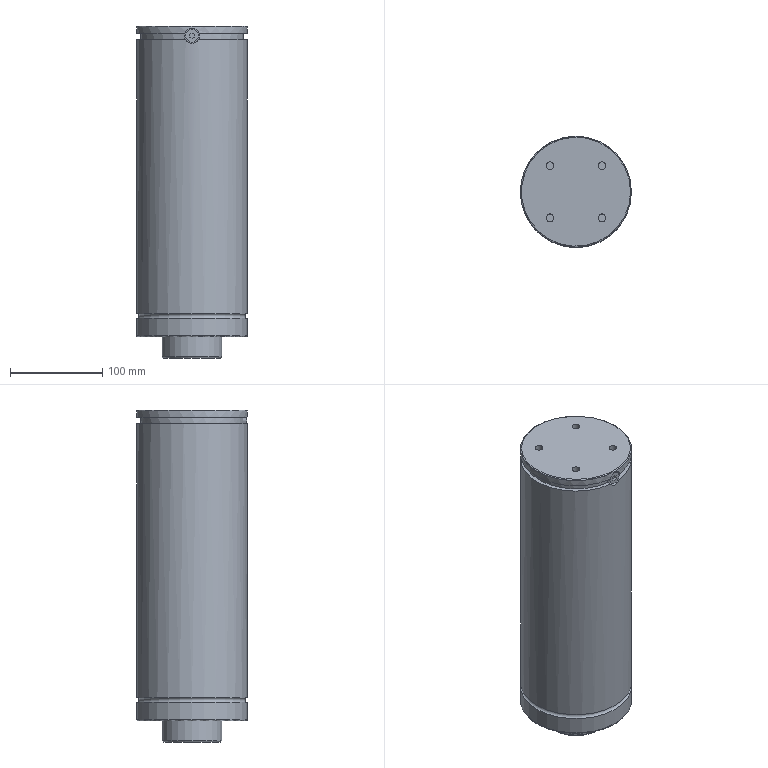Part | NX | features 1 2 | 1 solid | 38 faces | box 120.2 x 120.2 x 360 mm | volume 3879845 mm3 | plane 19 | cylinder 13 | torus 4 | cone 2 | commonest cylinder face diameters 8.4 x4 120.2 x3 6.6 x1 10 x1 14 x1 16.4 x1
STEP:
#1=CARTESIAN_POINT('',(2190.1,265.,32.15));
#2=VERTEX_POINT('',#1);
#3=CARTESIAN_POINT('',(2130.,265.,32.15));
#4=DIRECTION('',(0.,0.,1.));
#5=DIRECTION('',(1.,0.,0.));
#6=AXIS2_PLACEMENT_3D('',#3,#4,#5);
#7=CIRCLE('',#6,60.1);
#8=EDGE_CURVE('',#2,#2,#7,.T.);
#9=ORIENTED_EDGE('',*,*,#8,.F.);
#10=EDGE_LOOP('',(#9));
#11=FACE_BOUND('',#10,.T.);
#12=CARTESIAN_POINT('',(2190.1,265.,26.85));
#13=VERTEX_POINT('',#12);
#14=CARTESIAN_POINT('',(2130.,265.,26.85));
#15=DIRECTION('',(0.,0.,1.));
#16=DIRECTION('',(1.,0.,0.));
#17=AXIS2_PLACEMENT_3D('',#14,#15,#16);
#18=CIRCLE('',#17,60.1);
#19=EDGE_CURVE('',#13,#13,#18,.T.);
#20=ORIENTED_EDGE('',*,*,#19,.T.);
#21=EDGE_LOOP('',(#20));
#22=FACE_BOUND('',#21,.T.);
#23=CARTESIAN_POINT('',(2130.,265.,29.5));
#24=DIRECTION('',(0.,0.,-1.));
#25=DIRECTION('',(0.,-1.,0.));
#26=AXIS2_PLACEMENT_3D('',#23,#24,#25);
#27=TOROIDAL_SURFACE('',#26,60.1,2.65);
#28=ADVANCED_FACE('',(#11,#22),#27,.F.);
#29=CARTESIAN_POINT('',(2190.1,265.,8.));
#30=VERTEX_POINT('',#29);
#31=CARTESIAN_POINT('',(2130.,265.,8.));
#32=DIRECTION('',(0.,0.,1.));
#33=DIRECTION('',(1.,0.,0.));
#34=AXIS2_PLACEMENT_3D('',#31,#32,#33);
#35=CIRCLE('',#34,60.1);
#36=EDGE_CURVE('',#30,#30,#35,.T.);
#37=ORIENTED_EDGE('',*,*,#36,.F.);
#38=EDGE_LOOP('',(#37));
#39=FACE_BOUND('',#38,.T.);
#40=CARTESIAN_POINT('',(2189.1,265.,7.));
#41=VERTEX_POINT('',#40);
#42=CARTESIAN_POINT('',(2130.,265.,7.));
#43=DIRECTION('',(0.,0.,1.));
#44=DIRECTION('',(1.,0.,0.));
#45=AXIS2_PLACEMENT_3D('',#42,#43,#44);
#46=CIRCLE('',#45,59.1);
#47=EDGE_CURVE('',#41,#41,#46,.T.);
#48=ORIENTED_EDGE('',*,*,#47,.T.);
#49=EDGE_LOOP('',(#48));
#50=FACE_BOUND('',#49,.T.);
#51=CARTESIAN_POINT('',(2130.,265.,8.));
#52=DIRECTION('',(0.,0.,-1.));
#53=DIRECTION('',(0.,-1.,0.));
#54=AXIS2_PLACEMENT_3D('',#51,#52,#53);
#55=TOROIDAL_SURFACE('',#54,59.1,1.);
#56=ADVANCED_FACE('',(#39,#50),#55,.T.);
#57=ORIENTED_EDGE('',*,*,#19,.F.);
#58=EDGE_LOOP('',(#57));
#59=FACE_BOUND('',#58,.T.);
#60=ORIENTED_EDGE('',*,*,#36,.T.);
#61=EDGE_LOOP('',(#60));
#62=FACE_BOUND('',#61,.T.);
#63=CARTESIAN_POINT('',(2130.,265.,17.425));
#64=DIRECTION('',(0.,0.,1.));
#65=DIRECTION('',(0.,1.,0.));
#66=AXIS2_PLACEMENT_3D('',#63,#64,#65);
#67=CYLINDRICAL_SURFACE('',#66,60.1);
#68=ADVANCED_FACE('',(#59,#62),#67,.T.);
#69=CARTESIAN_POINT('',(2136.855,209.623,329.));
#70=VERTEX_POINT('',#69);
#71=CARTESIAN_POINT('',(2123.145,209.623,329.));
#72=VERTEX_POINT('',#71);
#73=CARTESIAN_POINT('',(2130.,265.,329.));
#74=DIRECTION('',(0.,0.,1.));
#75=DIRECTION('',(1.,0.,0.));
#76=AXIS2_PLACEMENT_3D('',#73,#74,#75);
#77=CIRCLE('',#76,55.8);
#78=EDGE_CURVE('',#70,#72,#77,.T.);
#79=ORIENTED_EDGE('',*,*,#78,.T.);
#80=CARTESIAN_POINT('',(2122.19,209.749,336.));
#81=VERTEX_POINT('',#80);
#82=CARTESIAN_POINT('',(2122.19,209.749,336.));
#83=CARTESIAN_POINT('',(2121.442,209.855,333.663));
#84=CARTESIAN_POINT('',(2121.8,209.789,331.049));
#85=CARTESIAN_POINT('',(2123.145,209.623,329.));
#86=B_SPLINE_CURVE_WITH_KNOTS('',3,(#82,#83,#84,#85),.UNSPECIFIED.,.F.,.F.,(4,4),(0.,0.007265),.UNSPECIFIED.);
#87=EDGE_CURVE('',#81,#72,#86,.T.);
#88=ORIENTED_EDGE('',*,*,#87,.F.);
#89=CARTESIAN_POINT('',(2137.81,209.749,336.));
#90=VERTEX_POINT('',#89);
#91=CARTESIAN_POINT('',(2130.,265.,336.));
#92=DIRECTION('',(0.,0.,1.));
#93=DIRECTION('',(1.,0.,0.));
#94=AXIS2_PLACEMENT_3D('',#91,#92,#93);
#95=CIRCLE('',#94,55.8);
#96=EDGE_CURVE('',#90,#81,#95,.T.);
#97=ORIENTED_EDGE('',*,*,#96,.F.);
#98=CARTESIAN_POINT('',(2136.855,209.623,329.));
#99=CARTESIAN_POINT('',(2138.2,209.789,331.049));
#100=CARTESIAN_POINT('',(2138.558,209.855,333.663));
#101=CARTESIAN_POINT('',(2137.81,209.749,336.));
#102=B_SPLINE_CURVE_WITH_KNOTS('',3,(#98,#99,#100,#101),.UNSPECIFIED.,.F.,.F.,(4,4),(0.,0.007265),.UNSPECIFIED.);
#103=EDGE_CURVE('',#70,#90,#102,.T.);
#104=ORIENTED_EDGE('',*,*,#103,.F.);
#105=EDGE_LOOP('',(#79,#88,#97,#104));
#106=FACE_BOUND('',#105,.T.);
#107=CARTESIAN_POINT('',(2130.,265.,332.5));
#108=DIRECTION('',(0.,0.,1.));
#109=DIRECTION('',(0.,1.,0.));
#110=AXIS2_PLACEMENT_3D('',#107,#108,#109);
#111=CYLINDRICAL_SURFACE('',#110,55.8);
#112=ADVANCED_FACE('',(#106),#111,.T.);
#113=CARTESIAN_POINT('',(2190.1,265.,343.));
#114=VERTEX_POINT('',#113);
#115=CARTESIAN_POINT('',(2130.,265.,343.));
#116=DIRECTION('',(0.,0.,1.));
#117=DIRECTION('',(1.,0.,0.));
#118=AXIS2_PLACEMENT_3D('',#115,#116,#117);
#119=CIRCLE('',#118,60.1);
#120=EDGE_CURVE('',#114,#114,#119,.T.);
#121=ORIENTED_EDGE('',*,*,#120,.F.);
#122=EDGE_LOOP('',(#121));
#123=FACE_BOUND('',#122,.T.);
#124=CARTESIAN_POINT('',(2137.81,205.41,336.));
#125=VERTEX_POINT('',#124);
#126=CARTESIAN_POINT('',(2122.19,205.41,336.));
#127=VERTEX_POINT('',#126);
#128=CARTESIAN_POINT('',(2130.,265.,336.));
#129=DIRECTION('',(0.,0.,1.));
#130=DIRECTION('',(1.,0.,0.));
#131=AXIS2_PLACEMENT_3D('',#128,#129,#130);
#132=CIRCLE('',#131,60.1);
#133=EDGE_CURVE('',#125,#127,#132,.T.);
#134=ORIENTED_EDGE('',*,*,#133,.T.);
#135=CARTESIAN_POINT('',(2137.81,205.41,336.));
#136=CARTESIAN_POINT('',(2137.279,205.34,337.657));
#137=CARTESIAN_POINT('',(2135.182,205.071,340.559));
#138=CARTESIAN_POINT('',(2129.995,204.815,342.267));
#139=CARTESIAN_POINT('',(2124.839,205.069,340.572));
#140=CARTESIAN_POINT('',(2122.721,205.34,337.657));
#141=CARTESIAN_POINT('',(2122.19,205.41,336.));
#142=B_SPLINE_CURVE_WITH_KNOTS('',3,(#135,#136,#137,#138,#139,#140,#141),.UNSPECIFIED.,.F.,.F.,(4,1,1,1,4),(-0.0103,-0.005148,-0.000000175,0.005148,0.0103),.UNSPECIFIED.);
#143=EDGE_CURVE('',#125,#127,#142,.T.);
#144=ORIENTED_EDGE('',*,*,#143,.F.);
#145=EDGE_LOOP('',(#134,#144));
#146=FACE_BOUND('',#145,.T.);
#147=CARTESIAN_POINT('',(2130.,265.,339.5));
#148=DIRECTION('',(0.,0.,1.));
#149=DIRECTION('',(0.,1.,0.));
#150=AXIS2_PLACEMENT_3D('',#147,#148,#149);
#151=CYLINDRICAL_SURFACE('',#150,60.1);
#152=ADVANCED_FACE('',(#123,#146),#151,.T.);
#153=CARTESIAN_POINT('',(2189.1,265.,344.));
#154=VERTEX_POINT('',#153);
#155=CARTESIAN_POINT('',(2130.,265.,344.));
#156=DIRECTION('',(0.,0.,1.));
#157=DIRECTION('',(1.,0.,0.));
#158=AXIS2_PLACEMENT_3D('',#155,#156,#157);
#159=CIRCLE('',#158,59.1);
#160=EDGE_CURVE('',#154,#154,#159,.T.);
#161=ORIENTED_EDGE('',*,*,#160,.F.);
#162=EDGE_LOOP('',(#161));
#163=FACE_BOUND('',#162,.T.);
#164=ORIENTED_EDGE('',*,*,#120,.T.);
#165=EDGE_LOOP('',(#164));
#166=FACE_BOUND('',#165,.T.);
#167=CARTESIAN_POINT('',(2130.,265.,343.));
#168=DIRECTION('',(0.,0.,-1.));
#169=DIRECTION('',(0.,-1.,0.));
#170=AXIS2_PLACEMENT_3D('',#167,#168,#169);
#171=TOROIDAL_SURFACE('',#170,59.1,1.);
#172=ADVANCED_FACE('',(#163,#166),#171,.T.);
#173=CARTESIAN_POINT('',(2162.5,265.,-14.5));
#174=VERTEX_POINT('',#173);
#175=CARTESIAN_POINT('',(2130.,265.,-14.5));
#176=DIRECTION('',(0.,0.,1.));
#177=DIRECTION('',(1.,0.,0.));
#178=AXIS2_PLACEMENT_3D('',#175,#176,#177);
#179=CIRCLE('',#178,32.5);
#180=EDGE_CURVE('',#174,#174,#179,.T.);
#181=ORIENTED_EDGE('',*,*,#180,.F.);
#182=EDGE_LOOP('',(#181));
#183=FACE_BOUND('',#182,.T.);
#184=CARTESIAN_POINT('',(2161.,265.,-16.));
#185=VERTEX_POINT('',#184);
#186=CARTESIAN_POINT('',(2130.,265.,-16.));
#187=DIRECTION('',(0.,0.,1.));
#188=DIRECTION('',(1.,0.,0.));
#189=AXIS2_PLACEMENT_3D('',#186,#187,#188);
#190=CIRCLE('',#189,31.);
#191=EDGE_CURVE('',#185,#185,#190,.T.);
#192=ORIENTED_EDGE('',*,*,#191,.T.);
#193=EDGE_LOOP('',(#192));
#194=FACE_BOUND('',#193,.T.);
#195=CARTESIAN_POINT('',(2130.,265.,-14.5));
#196=DIRECTION('',(0.,0.,-1.));
#197=DIRECTION('',(0.,-1.,0.));
#198=AXIS2_PLACEMENT_3D('',#195,#196,#197);
#199=TOROIDAL_SURFACE('',#198,31.,1.5);
#200=ADVANCED_FACE('',(#183,#194),#199,.T.);
#201=CARTESIAN_POINT('',(2162.5,265.,7.));
#202=VERTEX_POINT('',#201);
#203=CARTESIAN_POINT('',(2130.,265.,7.));
#204=DIRECTION('',(0.,0.,-1.));
#205=DIRECTION('',(1.,0.,0.));
#206=AXIS2_PLACEMENT_3D('',#203,#204,#205);
#207=CIRCLE('',#206,32.5);
#208=EDGE_CURVE('',#202,#202,#207,.T.);
#209=ORIENTED_EDGE('',*,*,#208,.T.);
#210=EDGE_LOOP('',(#209));
#211=FACE_BOUND('',#210,.T.);
#212=ORIENTED_EDGE('',*,*,#180,.T.);
#213=EDGE_LOOP('',(#212));
#214=FACE_BOUND('',#213,.T.);
#215=CARTESIAN_POINT('',(2130.,265.,-3.75));
#216=DIRECTION('',(0.,0.,1.));
#217=DIRECTION('',(0.,1.,0.));
#218=AXIS2_PLACEMENT_3D('',#215,#216,#217);
#219=CYLINDRICAL_SURFACE('',#218,32.5);
#220=ADVANCED_FACE('',(#211,#214),#219,.T.);
#221=CARTESIAN_POINT('',(2136.855,205.292,329.));
#222=VERTEX_POINT('',#221);
#223=CARTESIAN_POINT('',(2123.145,205.292,329.));
#224=VERTEX_POINT('',#223);
#225=CARTESIAN_POINT('',(2130.,265.,329.));
#226=DIRECTION('',(0.,0.,1.));
#227=DIRECTION('',(1.,0.,0.));
#228=AXIS2_PLACEMENT_3D('',#225,#226,#227);
#229=CIRCLE('',#228,60.1);
#230=EDGE_CURVE('',#222,#224,#229,.T.);
#231=ORIENTED_EDGE('',*,*,#230,.F.);
#232=CARTESIAN_POINT('',(2123.145,205.292,329.));
#233=CARTESIAN_POINT('',(2123.894,205.206,327.859));
#234=CARTESIAN_POINT('',(2125.933,205.,325.992));
#235=CARTESIAN_POINT('',(2130.001,204.85,324.954));
#236=CARTESIAN_POINT('',(2134.063,205.,325.991));
#237=CARTESIAN_POINT('',(2136.106,205.206,327.859));
#238=CARTESIAN_POINT('',(2136.855,205.292,329.));
#239=B_SPLINE_CURVE_WITH_KNOTS('',3,(#232,#233,#234,#235,#236,#237,#238),.UNSPECIFIED.,.F.,.F.,(4,1,1,1,4),(-0.008087,-0.004043,-0.000000027,0.004043,0.008087),.UNSPECIFIED.);
#240=EDGE_CURVE('',#224,#222,#239,.T.);
#241=ORIENTED_EDGE('',*,*,#240,.F.);
#242=EDGE_LOOP('',(#231,#241));
#243=FACE_BOUND('',#242,.T.);
#244=ORIENTED_EDGE('',*,*,#8,.T.);
#245=EDGE_LOOP('',(#244));
#246=FACE_BOUND('',#245,.T.);
#247=CARTESIAN_POINT('',(2130.,265.,180.575));
#248=DIRECTION('',(0.,0.,1.));
#249=DIRECTION('',(0.,1.,0.));
#250=AXIS2_PLACEMENT_3D('',#247,#248,#249);
#251=CYLINDRICAL_SURFACE('',#250,60.1);
#252=ADVANCED_FACE('',(#243,#246),#251,.T.);
#253=CARTESIAN_POINT('',(2138.2,210.9,333.5));
#254=VERTEX_POINT('',#253);
#255=CARTESIAN_POINT('',(2130.,210.9,333.5));
#256=DIRECTION('',(0.,1.,0.));
#257=DIRECTION('',(1.,0.,0.));
#258=AXIS2_PLACEMENT_3D('',#255,#256,#257);
#259=CIRCLE('',#258,8.2);
#260=EDGE_CURVE('',#254,#254,#259,.T.);
#261=ORIENTED_EDGE('',*,*,#260,.T.);
#262=EDGE_LOOP('',(#261));
#263=FACE_BOUND('',#262,.T.);
#264=ORIENTED_EDGE('',*,*,#103,.T.);
#265=CARTESIAN_POINT('',(2137.81,207.9,336.));
#266=DIRECTION('',(0.,-1.,0.));
#267=VECTOR('',#266,1000.);
#268=LINE('',#265,#267);
#269=EDGE_CURVE('',#90,#125,#268,.T.);
#270=ORIENTED_EDGE('',*,*,#269,.T.);
#271=ORIENTED_EDGE('',*,*,#143,.T.);
#272=CARTESIAN_POINT('',(2122.19,207.9,336.));
#273=DIRECTION('',(0.,1.,0.));
#274=VECTOR('',#273,1000.);
#275=LINE('',#272,#274);
#276=EDGE_CURVE('',#127,#81,#275,.T.);
#277=ORIENTED_EDGE('',*,*,#276,.T.);
#278=ORIENTED_EDGE('',*,*,#87,.T.);
#279=CARTESIAN_POINT('',(2123.145,207.9,329.));
#280=DIRECTION('',(0.,-1.,0.));
#281=VECTOR('',#280,1000.);
#282=LINE('',#279,#281);
#283=EDGE_CURVE('',#72,#224,#282,.T.);
#284=ORIENTED_EDGE('',*,*,#283,.T.);
#285=ORIENTED_EDGE('',*,*,#240,.T.);
#286=CARTESIAN_POINT('',(2136.855,207.9,329.));
#287=DIRECTION('',(0.,1.,0.));
#288=VECTOR('',#287,1000.);
#289=LINE('',#286,#288);
#290=EDGE_CURVE('',#222,#70,#289,.T.);
#291=ORIENTED_EDGE('',*,*,#290,.T.);
#292=EDGE_LOOP('',(#264,#270,#271,#277,#278,#284,#285,#291));
#293=FACE_BOUND('',#292,.T.);
#294=CARTESIAN_POINT('',(2130.,204.9,333.5));
#295=DIRECTION('',(0.,-1.,0.));
#296=DIRECTION('',(1.,0.,0.));
#297=AXIS2_PLACEMENT_3D('',#294,#295,#296);
#298=CYLINDRICAL_SURFACE('',#297,8.2);
#299=ADVANCED_FACE('',(#263,#293),#298,.F.);
#300=CARTESIAN_POINT('',(2105.916,293.284,324.));
#301=VERTEX_POINT('',#300);
#302=CARTESIAN_POINT('',(2101.716,293.284,324.));
#303=DIRECTION('',(0.,0.,-1.));
#304=DIRECTION('',(1.,0.,0.));
#305=AXIS2_PLACEMENT_3D('',#302,#303,#304);
#306=CIRCLE('',#305,4.2);
#307=EDGE_CURVE('',#301,#301,#306,.T.);
#308=ORIENTED_EDGE('',*,*,#307,.T.);
#309=EDGE_LOOP('',(#308));
#310=FACE_BOUND('',#309,.T.);
#311=CARTESIAN_POINT('',(2105.916,293.284,344.));
#312=VERTEX_POINT('',#311);
#313=CARTESIAN_POINT('',(2101.716,293.284,344.));
#314=DIRECTION('',(0.,0.,1.));
#315=DIRECTION('',(1.,0.,0.));
#316=AXIS2_PLACEMENT_3D('',#313,#314,#315);
#317=CIRCLE('',#316,4.2);
#318=EDGE_CURVE('',#312,#312,#317,.T.);
#319=ORIENTED_EDGE('',*,*,#318,.T.);
#320=EDGE_LOOP('',(#319));
#321=FACE_BOUND('',#320,.T.);
#322=CARTESIAN_POINT('',(2101.716,293.284,344.));
#323=DIRECTION('',(0.,0.,1.));
#324=DIRECTION('',(0.,1.,0.));
#325=AXIS2_PLACEMENT_3D('',#322,#323,#324);
#326=CYLINDRICAL_SURFACE('',#325,4.2);
#327=ADVANCED_FACE('',(#310,#321),#326,.F.);
#328=CARTESIAN_POINT('',(2162.484,293.284,324.));
#329=VERTEX_POINT('',#328);
#330=CARTESIAN_POINT('',(2158.284,293.284,324.));
#331=DIRECTION('',(0.,0.,-1.));
#332=DIRECTION('',(1.,0.,0.));
#333=AXIS2_PLACEMENT_3D('',#330,#331,#332);
#334=CIRCLE('',#333,4.2);
#335=EDGE_CURVE('',#329,#329,#334,.T.);
#336=ORIENTED_EDGE('',*,*,#335,.T.);
#337=EDGE_LOOP('',(#336));
#338=FACE_BOUND('',#337,.T.);
#339=CARTESIAN_POINT('',(2162.484,293.284,344.));
#340=VERTEX_POINT('',#339);
#341=CARTESIAN_POINT('',(2158.284,293.284,344.));
#342=DIRECTION('',(0.,0.,1.));
#343=DIRECTION('',(1.,0.,0.));
#344=AXIS2_PLACEMENT_3D('',#341,#342,#343);
#345=CIRCLE('',#344,4.2);
#346=EDGE_CURVE('',#340,#340,#345,.T.);
#347=ORIENTED_EDGE('',*,*,#346,.T.);
#348=EDGE_LOOP('',(#347));
#349=FACE_BOUND('',#348,.T.);
#350=CARTESIAN_POINT('',(2158.284,293.284,344.));
#351=DIRECTION('',(0.,0.,1.));
#352=DIRECTION('',(0.,1.,0.));
#353=AXIS2_PLACEMENT_3D('',#350,#351,#352);
#354=CYLINDRICAL_SURFACE('',#353,4.2);
#355=ADVANCED_FACE('',(#338,#349),#354,.F.);
#356=CARTESIAN_POINT('',(2162.484,236.716,324.));
#357=VERTEX_POINT('',#356);
#358=CARTESIAN_POINT('',(2158.284,236.716,324.));
#359=DIRECTION('',(0.,0.,-1.));
#360=DIRECTION('',(1.,0.,0.));
#361=AXIS2_PLACEMENT_3D('',#358,#359,#360);
#362=CIRCLE('',#361,4.2);
#363=EDGE_CURVE('',#357,#357,#362,.T.);
#364=ORIENTED_EDGE('',*,*,#363,.T.);
#365=EDGE_LOOP('',(#364));
#366=FACE_BOUND('',#365,.T.);
#367=CARTESIAN_POINT('',(2162.484,236.716,344.));
#368=VERTEX_POINT('',#367);
#369=CARTESIAN_POINT('',(2158.284,236.716,344.));
#370=DIRECTION('',(0.,0.,1.));
#371=DIRECTION('',(1.,0.,0.));
#372=AXIS2_PLACEMENT_3D('',#369,#370,#371);
#373=CIRCLE('',#372,4.2);
#374=EDGE_CURVE('',#368,#368,#373,.T.);
#375=ORIENTED_EDGE('',*,*,#374,.T.);
#376=EDGE_LOOP('',(#375));
#377=FACE_BOUND('',#376,.T.);
#378=CARTESIAN_POINT('',(2158.284,236.716,344.));
#379=DIRECTION('',(0.,0.,1.));
#380=DIRECTION('',(0.,1.,0.));
#381=AXIS2_PLACEMENT_3D('',#378,#379,#380);
#382=CYLINDRICAL_SURFACE('',#381,4.2);
#383=ADVANCED_FACE('',(#366,#377),#382,.F.);
#384=CARTESIAN_POINT('',(2105.916,236.716,324.));
#385=VERTEX_POINT('',#384);
#386=CARTESIAN_POINT('',(2101.716,236.716,324.));
#387=DIRECTION('',(0.,0.,-1.));
#388=DIRECTION('',(1.,0.,0.));
#389=AXIS2_PLACEMENT_3D('',#386,#387,#388);
#390=CIRCLE('',#389,4.2);
#391=EDGE_CURVE('',#385,#385,#390,.T.);
#392=ORIENTED_EDGE('',*,*,#391,.T.);
#393=EDGE_LOOP('',(#392));
#394=FACE_BOUND('',#393,.T.);
#395=CARTESIAN_POINT('',(2105.916,236.716,344.));
#396=VERTEX_POINT('',#395);
#397=CARTESIAN_POINT('',(2101.716,236.716,344.));
#398=DIRECTION('',(0.,0.,1.));
#399=DIRECTION('',(1.,0.,0.));
#400=AXIS2_PLACEMENT_3D('',#397,#398,#399);
#401=CIRCLE('',#400,4.2);
#402=EDGE_CURVE('',#396,#396,#401,.T.);
#403=ORIENTED_EDGE('',*,*,#402,.T.);
#404=EDGE_LOOP('',(#403));
#405=FACE_BOUND('',#404,.T.);
#406=CARTESIAN_POINT('',(2101.716,236.716,344.));
#407=DIRECTION('',(0.,0.,1.));
#408=DIRECTION('',(0.,1.,0.));
#409=AXIS2_PLACEMENT_3D('',#406,#407,#408);
#410=CYLINDRICAL_SURFACE('',#409,4.2);
#411=ADVANCED_FACE('',(#394,#405),#410,.F.);
#412=CARTESIAN_POINT('',(2137.,210.9,333.5));
#413=VERTEX_POINT('',#412);
#414=CARTESIAN_POINT('',(2130.,210.9,333.5));
#415=DIRECTION('',(0.,-1.,0.));
#416=DIRECTION('',(1.,0.,0.));
#417=AXIS2_PLACEMENT_3D('',#414,#415,#416);
#418=CIRCLE('',#417,7.);
#419=EDGE_CURVE('',#413,#413,#418,.T.);
#420=ORIENTED_EDGE('',*,*,#419,.T.);
#421=EDGE_LOOP('',(#420));
#422=FACE_BOUND('',#421,.T.);
#423=CARTESIAN_POINT('',(2137.,205.9,333.5));
#424=VERTEX_POINT('',#423);
#425=CARTESIAN_POINT('',(2130.,205.9,333.5));
#426=DIRECTION('',(0.,-1.,0.));
#427=DIRECTION('',(1.,0.,0.));
#428=AXIS2_PLACEMENT_3D('',#425,#426,#427);
#429=CIRCLE('',#428,7.);
#430=EDGE_CURVE('',#424,#424,#429,.T.);
#431=ORIENTED_EDGE('',*,*,#430,.F.);
#432=EDGE_LOOP('',(#431));
#433=FACE_BOUND('',#432,.T.);
#434=CARTESIAN_POINT('',(2130.,265.,333.5));
#435=DIRECTION('',(0.,1.,0.));
#436=DIRECTION('',(-1.,0.,0.));
#437=AXIS2_PLACEMENT_3D('',#434,#435,#436);
#438=CYLINDRICAL_SURFACE('',#437,7.);
#439=ADVANCED_FACE('',(#422,#433),#438,.T.);
#440=CARTESIAN_POINT('',(2130.,270.5,-16.));
#441=VERTEX_POINT('',#440);
#442=CARTESIAN_POINT('',(2130.,265.,-16.));
#443=DIRECTION('',(0.,0.,-1.));
#444=DIRECTION('',(0.,1.,0.));
#445=AXIS2_PLACEMENT_3D('',#442,#443,#444);
#446=CIRCLE('',#445,5.5);
#447=EDGE_CURVE('',#441,#441,#446,.T.);
#448=ORIENTED_EDGE('',*,*,#447,.T.);
#449=EDGE_LOOP('',(#448));
#450=FACE_BOUND('',#449,.T.);
#451=CARTESIAN_POINT('',(2130.,270.,-15.));
#452=VERTEX_POINT('',#451);
#453=CARTESIAN_POINT('',(2130.,265.,-15.));
#454=DIRECTION('',(0.,0.,1.));
#455=DIRECTION('',(0.,1.,0.));
#456=AXIS2_PLACEMENT_3D('',#453,#454,#455);
#457=CIRCLE('',#456,5.);
#458=EDGE_CURVE('',#452,#452,#457,.T.);
#459=ORIENTED_EDGE('',*,*,#458,.T.);
#460=EDGE_LOOP('',(#459));
#461=FACE_BOUND('',#460,.T.);
#462=CARTESIAN_POINT('',(2130.,265.,-15.5));
#463=DIRECTION('',(0.,0.,-1.));
#464=DIRECTION('',(0.,-1.,0.));
#465=AXIS2_PLACEMENT_3D('',#462,#463,#464);
#466=CONICAL_SURFACE('',#465,5.25,0.4636);
#467=ADVANCED_FACE('',(#450,#461),#466,.F.);
#468=ORIENTED_EDGE('',*,*,#458,.F.);
#469=EDGE_LOOP('',(#468));
#470=FACE_BOUND('',#469,.T.);
#471=CARTESIAN_POINT('',(2130.,270.,-10.));
#472=VERTEX_POINT('',#471);
#473=CARTESIAN_POINT('',(2130.,265.,-10.));
#474=DIRECTION('',(0.,0.,1.));
#475=DIRECTION('',(0.,1.,0.));
#476=AXIS2_PLACEMENT_3D('',#473,#474,#475);
#477=CIRCLE('',#476,5.);
#478=EDGE_CURVE('',#472,#472,#477,.T.);
#479=ORIENTED_EDGE('',*,*,#478,.T.);
#480=EDGE_LOOP('',(#479));
#481=FACE_BOUND('',#480,.T.);
#482=CARTESIAN_POINT('',(2130.,265.,-12.5));
#483=DIRECTION('',(0.,0.,1.));
#484=DIRECTION('',(0.,1.,0.));
#485=AXIS2_PLACEMENT_3D('',#482,#483,#484);
#486=CYLINDRICAL_SURFACE('',#485,5.);
#487=ADVANCED_FACE('',(#470,#481),#486,.F.);
#488=CARTESIAN_POINT('',(2130.,268.3,-10.));
#489=VERTEX_POINT('',#488);
#490=CARTESIAN_POINT('',(2130.,265.,-10.));
#491=DIRECTION('',(0.,0.,1.));
#492=DIRECTION('',(0.,1.,0.));
#493=AXIS2_PLACEMENT_3D('',#490,#491,#492);
#494=CIRCLE('',#493,3.3);
#495=EDGE_CURVE('',#489,#489,#494,.T.);
#496=ORIENTED_EDGE('',*,*,#495,.F.);
#497=EDGE_LOOP('',(#496));
#498=FACE_BOUND('',#497,.T.);
#499=CARTESIAN_POINT('',(2130.,268.3,-2.));
#500=VERTEX_POINT('',#499);
#501=CARTESIAN_POINT('',(2130.,265.,-2.));
#502=DIRECTION('',(0.,0.,1.));
#503=DIRECTION('',(0.,1.,0.));
#504=AXIS2_PLACEMENT_3D('',#501,#502,#503);
#505=CIRCLE('',#504,3.3);
#506=EDGE_CURVE('',#500,#500,#505,.T.);
#507=ORIENTED_EDGE('',*,*,#506,.T.);
#508=EDGE_LOOP('',(#507));
#509=FACE_BOUND('',#508,.T.);
#510=CARTESIAN_POINT('',(2130.,265.,-6.));
#511=DIRECTION('',(0.,0.,1.));
#512=DIRECTION('',(0.,1.,0.));
#513=AXIS2_PLACEMENT_3D('',#510,#511,#512);
#514=CYLINDRICAL_SURFACE('',#513,3.3);
#515=ADVANCED_FACE('',(#498,#509),#514,.F.);
#516=CARTESIAN_POINT('',(2130.,265.,0.));
#517=VERTEX_POINT('',#516);
#518=VERTEX_LOOP('',#517);
#519=FACE_BOUND('',#518,.T.);
#520=ORIENTED_EDGE('',*,*,#506,.F.);
#521=EDGE_LOOP('',(#520));
#522=FACE_BOUND('',#521,.T.);
#523=CARTESIAN_POINT('',(2130.,265.,-1.));
#524=DIRECTION('',(0.,0.,-1.));
#525=DIRECTION('',(0.,-1.,0.));
#526=AXIS2_PLACEMENT_3D('',#523,#524,#525);
#527=CONICAL_SURFACE('',#526,1.65,1.026);
#528=ADVANCED_FACE('',(#519,#522),#527,.F.);
#529=ORIENTED_EDGE('',*,*,#478,.F.);
#530=EDGE_LOOP('',(#529));
#531=FACE_BOUND('',#530,.T.);
#532=ORIENTED_EDGE('',*,*,#495,.T.);
#533=EDGE_LOOP('',(#532));
#534=FACE_BOUND('',#533,.T.);
#535=CARTESIAN_POINT('',(2130.,269.15,-10.));
#536=DIRECTION('',(0.,0.,1.));
#537=DIRECTION('',(0.,1.,0.));
#538=AXIS2_PLACEMENT_3D('',#535,#536,#537);
#539=PLANE('',#538);
#540=ADVANCED_FACE('',(#531,#534),#539,.F.);
#541=CARTESIAN_POINT('',(2130.,205.9,330.613));
#542=VERTEX_POINT('',#541);
#543=CARTESIAN_POINT('',(2132.5,205.9,332.057));
#544=VERTEX_POINT('',#543);
#545=CARTESIAN_POINT('',(2134.148,205.9,333.008));
#546=DIRECTION('',(0.866,0.,0.5));
#547=VECTOR('',#546,1000.);
#548=LINE('',#545,#547);
#549=EDGE_CURVE('',#542,#544,#548,.T.);
#550=ORIENTED_EDGE('',*,*,#549,.T.);
#551=CARTESIAN_POINT('',(2132.5,208.9,332.057));
#552=VERTEX_POINT('',#551);
#553=CARTESIAN_POINT('',(2132.5,204.9,332.057));
#554=DIRECTION('',(0.,1.,0.));
#555=VECTOR('',#554,1000.);
#556=LINE('',#553,#555);
#557=EDGE_CURVE('',#544,#552,#556,.T.);
#558=ORIENTED_EDGE('',*,*,#557,.T.);
#559=CARTESIAN_POINT('',(2130.,208.9,330.613));
#560=VERTEX_POINT('',#559);
#561=CARTESIAN_POINT('',(2132.5,208.9,332.057));
#562=DIRECTION('',(-0.866,0.,-0.5));
#563=VECTOR('',#562,1000.);
#564=LINE('',#561,#563);
#565=EDGE_CURVE('',#552,#560,#564,.T.);
#566=ORIENTED_EDGE('',*,*,#565,.T.);
#567=CARTESIAN_POINT('',(2130.,204.9,330.613));
#568=DIRECTION('',(0.,1.,0.));
#569=VECTOR('',#568,1000.);
#570=LINE('',#567,#569);
#571=EDGE_CURVE('',#542,#560,#570,.T.);
#572=ORIENTED_EDGE('',*,*,#571,.F.);
#573=EDGE_LOOP('',(#550,#558,#566,#572));
#574=FACE_BOUND('',#573,.T.);
#575=CARTESIAN_POINT('',(2132.5,204.9,332.057));
#576=DIRECTION('',(0.5,0.,-0.866));
#577=DIRECTION('',(-0.866,0.,-0.5));
#578=AXIS2_PLACEMENT_3D('',#575,#576,#577);
#579=PLANE('',#578);
#580=ADVANCED_FACE('',(#574),#579,.F.);
#581=CARTESIAN_POINT('',(2132.5,205.9,334.943));
#582=VERTEX_POINT('',#581);
#583=CARTESIAN_POINT('',(2132.5,205.9,339.472));
#584=DIRECTION('',(0.,0.,1.));
#585=VECTOR('',#584,1000.);
#586=LINE('',#583,#585);
#587=EDGE_CURVE('',#544,#582,#586,.T.);
#588=ORIENTED_EDGE('',*,*,#587,.T.);
#589=CARTESIAN_POINT('',(2132.5,208.9,334.943));
#590=VERTEX_POINT('',#589);
#591=CARTESIAN_POINT('',(2132.5,204.9,334.943));
#592=DIRECTION('',(0.,1.,0.));
#593=VECTOR('',#592,1000.);
#594=LINE('',#591,#593);
#595=EDGE_CURVE('',#582,#590,#594,.T.);
#596=ORIENTED_EDGE('',*,*,#595,.T.);
#597=CARTESIAN_POINT('',(2132.5,208.9,334.943));
#598=DIRECTION('',(0.,0.,-1.));
#599=VECTOR('',#598,1000.);
#600=LINE('',#597,#599);
#601=EDGE_CURVE('',#590,#552,#600,.T.);
#602=ORIENTED_EDGE('',*,*,#601,.T.);
#603=ORIENTED_EDGE('',*,*,#557,.F.);
#604=EDGE_LOOP('',(#588,#596,#602,#603));
#605=FACE_BOUND('',#604,.T.);
#606=CARTESIAN_POINT('',(2132.5,204.9,334.943));
#607=DIRECTION('',(1.,0.,0.));
#608=DIRECTION('',(0.,1.,0.));
#609=AXIS2_PLACEMENT_3D('',#606,#607,#608);
#610=PLANE('',#609);
#611=ADVANCED_FACE('',(#605),#610,.F.);
#612=CARTESIAN_POINT('',(2130.,205.9,336.387));
#613=VERTEX_POINT('',#612);
#614=CARTESIAN_POINT('',(2128.352,205.9,337.338));
#615=DIRECTION('',(-0.866,0.,0.5));
#616=VECTOR('',#615,1000.);
#617=LINE('',#614,#616);
#618=EDGE_CURVE('',#582,#613,#617,.T.);
#619=ORIENTED_EDGE('',*,*,#618,.T.);
#620=CARTESIAN_POINT('',(2130.,208.9,336.387));
#621=VERTEX_POINT('',#620);
#622=CARTESIAN_POINT('',(2130.,204.9,336.387));
#623=DIRECTION('',(0.,1.,0.));
#624=VECTOR('',#623,1000.);
#625=LINE('',#622,#624);
#626=EDGE_CURVE('',#613,#621,#625,.T.);
#627=ORIENTED_EDGE('',*,*,#626,.T.);
#628=CARTESIAN_POINT('',(2130.,208.9,336.387));
#629=DIRECTION('',(0.866,0.,-0.5));
#630=VECTOR('',#629,1000.);
#631=LINE('',#628,#630);
#632=EDGE_CURVE('',#621,#590,#631,.T.);
#633=ORIENTED_EDGE('',*,*,#632,.T.);
#634=ORIENTED_EDGE('',*,*,#595,.F.);
#635=EDGE_LOOP('',(#619,#627,#633,#634));
#636=FACE_BOUND('',#635,.T.);
#637=CARTESIAN_POINT('',(2130.,204.9,336.387));
#638=DIRECTION('',(0.5,0.,0.866));
#639=DIRECTION('',(0.866,0.,-0.5));
#640=AXIS2_PLACEMENT_3D('',#637,#638,#639);
#641=PLANE('',#640);
#642=ADVANCED_FACE('',(#636),#641,.F.);
#643=CARTESIAN_POINT('',(2127.5,205.9,334.943));
#644=VERTEX_POINT('',#643);
#645=CARTESIAN_POINT('',(2130.398,205.9,336.617));
#646=DIRECTION('',(-0.866,0.,-0.5));
#647=VECTOR('',#646,1000.);
#648=LINE('',#645,#647);
#649=EDGE_CURVE('',#613,#644,#648,.T.);
#650=ORIENTED_EDGE('',*,*,#649,.T.);
#651=CARTESIAN_POINT('',(2127.5,208.9,334.943));
#652=VERTEX_POINT('',#651);
#653=CARTESIAN_POINT('',(2127.5,204.9,334.943));
#654=DIRECTION('',(0.,1.,0.));
#655=VECTOR('',#654,1000.);
#656=LINE('',#653,#655);
#657=EDGE_CURVE('',#644,#652,#656,.T.);
#658=ORIENTED_EDGE('',*,*,#657,.T.);
#659=CARTESIAN_POINT('',(2127.5,208.9,334.943));
#660=DIRECTION('',(0.866,0.,0.5));
#661=VECTOR('',#660,1000.);
#662=LINE('',#659,#661);
#663=EDGE_CURVE('',#652,#621,#662,.T.);
#664=ORIENTED_EDGE('',*,*,#663,.T.);
#665=ORIENTED_EDGE('',*,*,#626,.F.);
#666=EDGE_LOOP('',(#650,#658,#664,#665));
#667=FACE_BOUND('',#666,.T.);
#668=CARTESIAN_POINT('',(2127.5,204.9,334.943));
#669=DIRECTION('',(-0.5,0.,0.866));
#670=DIRECTION('',(0.866,0.,0.5));
#671=AXIS2_PLACEMENT_3D('',#668,#669,#670);
#672=PLANE('',#671);
#673=ADVANCED_FACE('',(#667),#672,.F.);
#674=CARTESIAN_POINT('',(2127.5,205.9,332.057));
#675=VERTEX_POINT('',#674);
#676=CARTESIAN_POINT('',(2127.102,205.9,332.287));
#677=DIRECTION('',(0.866,0.,-0.5));
#678=VECTOR('',#677,1000.);
#679=LINE('',#676,#678);
#680=EDGE_CURVE('',#675,#542,#679,.T.);
#681=ORIENTED_EDGE('',*,*,#680,.T.);
#682=ORIENTED_EDGE('',*,*,#571,.T.);
#683=CARTESIAN_POINT('',(2127.5,208.9,332.057));
#684=VERTEX_POINT('',#683);
#685=CARTESIAN_POINT('',(2130.,208.9,330.613));
#686=DIRECTION('',(-0.866,0.,0.5));
#687=VECTOR('',#686,1000.);
#688=LINE('',#685,#687);
#689=EDGE_CURVE('',#560,#684,#688,.T.);
#690=ORIENTED_EDGE('',*,*,#689,.T.);
#691=CARTESIAN_POINT('',(2127.5,204.9,332.057));
#692=DIRECTION('',(0.,1.,0.));
#693=VECTOR('',#692,1000.);
#694=LINE('',#691,#693);
#695=EDGE_CURVE('',#675,#684,#694,.T.);
#696=ORIENTED_EDGE('',*,*,#695,.F.);
#697=EDGE_LOOP('',(#681,#682,#690,#696));
#698=FACE_BOUND('',#697,.T.);
#699=CARTESIAN_POINT('',(2130.,204.9,330.613));
#700=DIRECTION('',(-0.5,0.,-0.866));
#701=DIRECTION('',(-0.866,0.,0.5));
#702=AXIS2_PLACEMENT_3D('',#699,#700,#701);
#703=PLANE('',#702);
#704=ADVANCED_FACE('',(#698),#703,.F.);
#705=CARTESIAN_POINT('',(2127.5,205.9,338.028));
#706=DIRECTION('',(0.,0.,-1.));
#707=VECTOR('',#706,1000.);
#708=LINE('',#705,#707);
#709=EDGE_CURVE('',#644,#675,#708,.T.);
#710=ORIENTED_EDGE('',*,*,#709,.T.);
#711=ORIENTED_EDGE('',*,*,#695,.T.);
#712=CARTESIAN_POINT('',(2127.5,208.9,332.057));
#713=DIRECTION('',(0.,0.,1.));
#714=VECTOR('',#713,1000.);
#715=LINE('',#712,#714);
#716=EDGE_CURVE('',#684,#652,#715,.T.);
#717=ORIENTED_EDGE('',*,*,#716,.T.);
#718=ORIENTED_EDGE('',*,*,#657,.F.);
#719=EDGE_LOOP('',(#710,#711,#717,#718));
#720=FACE_BOUND('',#719,.T.);
#721=CARTESIAN_POINT('',(2127.5,204.9,332.057));
#722=DIRECTION('',(-1.,0.,0.));
#723=DIRECTION('',(0.,-1.,0.));
#724=AXIS2_PLACEMENT_3D('',#721,#722,#723);
#725=PLANE('',#724);
#726=ADVANCED_FACE('',(#720),#725,.F.);
#727=ORIENTED_EDGE('',*,*,#663,.F.);
#728=ORIENTED_EDGE('',*,*,#716,.F.);
#729=ORIENTED_EDGE('',*,*,#689,.F.);
#730=ORIENTED_EDGE('',*,*,#565,.F.);
#731=ORIENTED_EDGE('',*,*,#601,.F.);
#732=ORIENTED_EDGE('',*,*,#632,.F.);
#733=EDGE_LOOP('',(#727,#728,#729,#730,#731,#732));
#734=FACE_BOUND('',#733,.T.);
#735=CARTESIAN_POINT('',(2130.,208.9,344.));
#736=DIRECTION('',(0.,-1.,0.));
#737=DIRECTION('',(1.,0.,0.));
#738=AXIS2_PLACEMENT_3D('',#735,#736,#737);
#739=PLANE('',#738);
#740=ADVANCED_FACE('',(#734),#739,.T.);
#741=ORIENTED_EDGE('',*,*,#649,.F.);
#742=ORIENTED_EDGE('',*,*,#618,.F.);
#743=ORIENTED_EDGE('',*,*,#587,.F.);
#744=ORIENTED_EDGE('',*,*,#549,.F.);
#745=ORIENTED_EDGE('',*,*,#680,.F.);
#746=ORIENTED_EDGE('',*,*,#709,.F.);
#747=EDGE_LOOP('',(#741,#742,#743,#744,#745,#746));
#748=FACE_BOUND('',#747,.T.);
#749=ORIENTED_EDGE('',*,*,#430,.T.);
#750=EDGE_LOOP('',(#749));
#751=FACE_BOUND('',#750,.T.);
#752=CARTESIAN_POINT('',(2130.,205.9,344.));
#753=DIRECTION('',(0.,-1.,0.));
#754=DIRECTION('',(1.,0.,0.));
#755=AXIS2_PLACEMENT_3D('',#752,#753,#754);
#756=PLANE('',#755);
#757=ADVANCED_FACE('',(#748,#751),#756,.T.);
#758=ORIENTED_EDGE('',*,*,#391,.F.);
#759=EDGE_LOOP('',(#758));
#760=FACE_BOUND('',#759,.T.);
#761=CARTESIAN_POINT('',(2130.,265.,324.));
#762=DIRECTION('',(0.,0.,-1.));
#763=DIRECTION('',(0.,-1.,0.));
#764=AXIS2_PLACEMENT_3D('',#761,#762,#763);
#765=PLANE('',#764);
#766=ADVANCED_FACE('',(#760),#765,.F.);
#767=ORIENTED_EDGE('',*,*,#363,.F.);
#768=EDGE_LOOP('',(#767));
#769=FACE_BOUND('',#768,.T.);
#770=CARTESIAN_POINT('',(2130.,265.,324.));
#771=DIRECTION('',(0.,0.,-1.));
#772=DIRECTION('',(0.,-1.,0.));
#773=AXIS2_PLACEMENT_3D('',#770,#771,#772);
#774=PLANE('',#773);
#775=ADVANCED_FACE('',(#769),#774,.F.);
#776=ORIENTED_EDGE('',*,*,#335,.F.);
#777=EDGE_LOOP('',(#776));
#778=FACE_BOUND('',#777,.T.);
#779=CARTESIAN_POINT('',(2130.,265.,324.));
#780=DIRECTION('',(0.,0.,-1.));
#781=DIRECTION('',(0.,-1.,0.));
#782=AXIS2_PLACEMENT_3D('',#779,#780,#781);
#783=PLANE('',#782);
#784=ADVANCED_FACE('',(#778),#783,.F.);
#785=ORIENTED_EDGE('',*,*,#307,.F.);
#786=EDGE_LOOP('',(#785));
#787=FACE_BOUND('',#786,.T.);
#788=CARTESIAN_POINT('',(2130.,265.,324.));
#789=DIRECTION('',(0.,0.,-1.));
#790=DIRECTION('',(0.,-1.,0.));
#791=AXIS2_PLACEMENT_3D('',#788,#789,#790);
#792=PLANE('',#791);
#793=ADVANCED_FACE('',(#787),#792,.F.);
#794=ORIENTED_EDGE('',*,*,#419,.F.);
#795=EDGE_LOOP('',(#794));
#796=FACE_BOUND('',#795,.T.);
#797=ORIENTED_EDGE('',*,*,#260,.F.);
#798=EDGE_LOOP('',(#797));
#799=FACE_BOUND('',#798,.T.);
#800=CARTESIAN_POINT('',(2130.,210.9,344.));
#801=DIRECTION('',(0.,-1.,0.));
#802=DIRECTION('',(1.,0.,0.));
#803=AXIS2_PLACEMENT_3D('',#800,#801,#802);
#804=PLANE('',#803);
#805=ADVANCED_FACE('',(#796,#799),#804,.T.);
#806=ORIENTED_EDGE('',*,*,#447,.F.);
#807=EDGE_LOOP('',(#806));
#808=FACE_BOUND('',#807,.T.);
#809=ORIENTED_EDGE('',*,*,#191,.F.);
#810=EDGE_LOOP('',(#809));
#811=FACE_BOUND('',#810,.T.);
#812=CARTESIAN_POINT('',(2145.5,265.,-16.));
#813=DIRECTION('',(0.,0.,-1.));
#814=DIRECTION('',(0.,-1.,0.));
#815=AXIS2_PLACEMENT_3D('',#812,#813,#814);
#816=PLANE('',#815);
#817=ADVANCED_FACE('',(#808,#811),#816,.T.);
#818=ORIENTED_EDGE('',*,*,#402,.F.);
#819=EDGE_LOOP('',(#818));
#820=FACE_BOUND('',#819,.T.);
#821=ORIENTED_EDGE('',*,*,#374,.F.);
#822=EDGE_LOOP('',(#821));
#823=FACE_BOUND('',#822,.T.);
#824=ORIENTED_EDGE('',*,*,#346,.F.);
#825=EDGE_LOOP('',(#824));
#826=FACE_BOUND('',#825,.T.);
#827=ORIENTED_EDGE('',*,*,#318,.F.);
#828=EDGE_LOOP('',(#827));
#829=FACE_BOUND('',#828,.T.);
#830=ORIENTED_EDGE('',*,*,#160,.T.);
#831=EDGE_LOOP('',(#830));
#832=FACE_BOUND('',#831,.T.);
#833=CARTESIAN_POINT('',(2159.55,265.,344.));
#834=DIRECTION('',(0.,0.,1.));
#835=DIRECTION('',(1.,0.,0.));
#836=AXIS2_PLACEMENT_3D('',#833,#834,#835);
#837=PLANE('',#836);
#838=ADVANCED_FACE('',(#820,#823,#826,#829,#832),#837,.T.);
#839=ORIENTED_EDGE('',*,*,#276,.F.);
#840=ORIENTED_EDGE('',*,*,#133,.F.);
#841=ORIENTED_EDGE('',*,*,#269,.F.);
#842=ORIENTED_EDGE('',*,*,#96,.T.);
#843=EDGE_LOOP('',(#839,#840,#841,#842));
#844=FACE_BOUND('',#843,.T.);
#845=CARTESIAN_POINT('',(2187.95,265.,336.));
#846=DIRECTION('',(0.,0.,-1.));
#847=DIRECTION('',(0.,-1.,0.));
#848=AXIS2_PLACEMENT_3D('',#845,#846,#847);
#849=PLANE('',#848);
#850=ADVANCED_FACE('',(#844),#849,.T.);
#851=ORIENTED_EDGE('',*,*,#283,.F.);
#852=ORIENTED_EDGE('',*,*,#78,.F.);
#853=ORIENTED_EDGE('',*,*,#290,.F.);
#854=ORIENTED_EDGE('',*,*,#230,.T.);
#855=EDGE_LOOP('',(#851,#852,#853,#854));
#856=FACE_BOUND('',#855,.T.);
#857=CARTESIAN_POINT('',(2187.95,265.,329.));
#858=DIRECTION('',(0.,0.,1.));
#859=DIRECTION('',(0.,1.,0.));
#860=AXIS2_PLACEMENT_3D('',#857,#858,#859);
#861=PLANE('',#860);
#862=ADVANCED_FACE('',(#856),#861,.T.);
#863=ORIENTED_EDGE('',*,*,#208,.F.);
#864=EDGE_LOOP('',(#863));
#865=FACE_BOUND('',#864,.T.);
#866=ORIENTED_EDGE('',*,*,#47,.F.);
#867=EDGE_LOOP('',(#866));
#868=FACE_BOUND('',#867,.T.);
#869=CARTESIAN_POINT('',(2159.55,265.,7.));
#870=DIRECTION('',(0.,0.,-1.));
#871=DIRECTION('',(0.,-1.,0.));
#872=AXIS2_PLACEMENT_3D('',#869,#870,#871);
#873=PLANE('',#872);
#874=ADVANCED_FACE('',(#865,#868),#873,.T.);
#875=CLOSED_SHELL('',(#28,#56,#68,#112,#152,#172,#200,#220,#252,#299,#327,#355,#383,#411,#439,#467,#487,#515,#528,#540,#580,#611,#642,#673,#704,#726,#740,#757,#766,#775,#784,#793,#805,#817,#838,#850,#862,#874));
#876=MANIFOLD_SOLID_BREP('',#875);
#877=(LENGTH_UNIT()NAMED_UNIT(*)SI_UNIT(.MILLI.,.METRE.));
#878=UNCERTAINTY_MEASURE_WITH_UNIT(LENGTH_MEASURE(0.0508),#877,'','');
#879=(NAMED_UNIT(*)PLANE_ANGLE_UNIT()SI_UNIT($,.RADIAN.));
#880=(NAMED_UNIT(*)SI_UNIT($,.STERADIAN.)SOLID_ANGLE_UNIT());
#881=(GEOMETRIC_REPRESENTATION_CONTEXT(3)GLOBAL_UNCERTAINTY_ASSIGNED_CONTEXT((#878))GLOBAL_UNIT_ASSIGNED_CONTEXT((#877,#879,#880))REPRESENTATION_CONTEXT('',''));
#882=ADVANCED_BREP_SHAPE_REPRESENTATION('',(#876),#881);